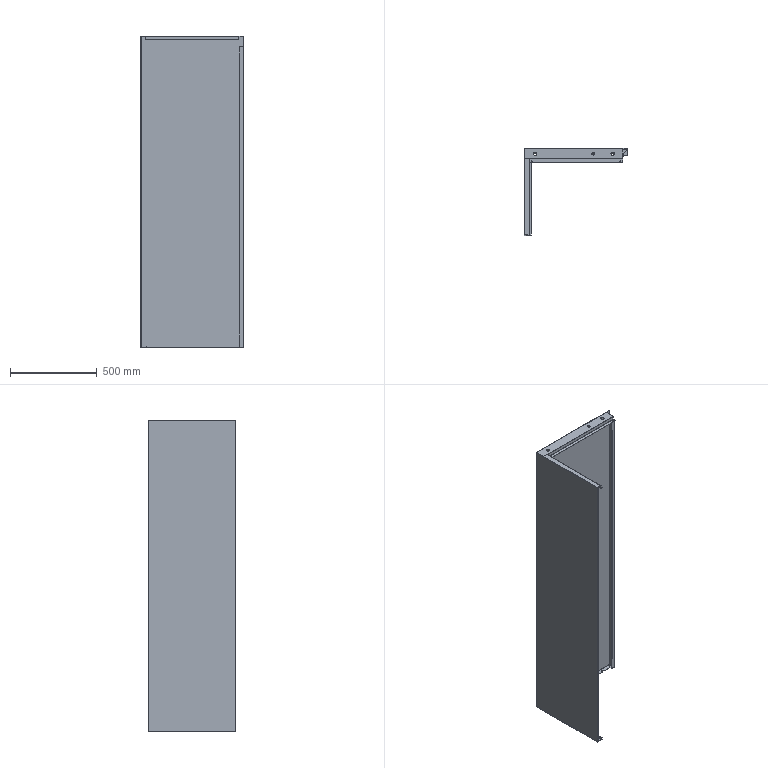Part | STEP file | 1 solid | 197 faces | box 600.001 x 500.001 x 1800 mm | volume 2227675 mm3 | plane 146 | cylinder 48 | spline 3 | commonest cylinder face diameters 0.4 x15 2.4 x15 18 x12 19 x4 16 x2